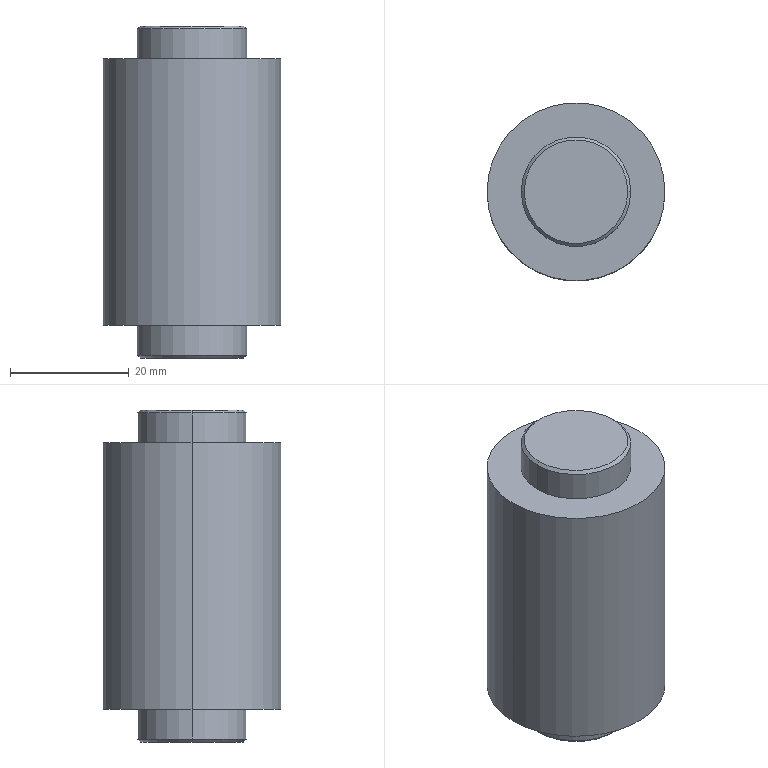Part | STEP file | CDAN75-Mbe | 1 solid | 14 faces | box 30 x 30 x 56 mm | volume 34751 mm3 | cylinder 6 | cone 4 | plane 4 | commonest cylinder face diameters 18.5 x4 30 x2
STEP:
#1=CARTESIAN_POINT('',(0.,0.,0.));
#2=DIRECTION('',(0.,0.,1.));
#3=DIRECTION('',(1.,0.,0.));
#4=AXIS2_PLACEMENT_3D('',#1,#2,#3);
#5=CARTESIAN_POINT('',(-71.,-59.,22.5));
#6=VERTEX_POINT('',#5);
#7=CARTESIAN_POINT('',(-41.,-59.,22.5));
#8=VERTEX_POINT('',#7);
#9=CARTESIAN_POINT('',(-56.,-59.,22.5));
#10=DIRECTION('',(0.,0.,-1.));
#11=DIRECTION('',(-1.,0.,0.));
#12=AXIS2_PLACEMENT_3D('',#9,#10,#11);
#13=CIRCLE('',#12,15.);
#14=CARTESIAN_POINT('',(-56.,-59.,0.));
#15=DIRECTION('',(0.,0.,-1.));
#16=DIRECTION('',(-1.,0.,0.));
#17=AXIS2_PLACEMENT_3D('',#14,#15,#16);
#18=CYLINDRICAL_SURFACE('',#17,15.);
#19=CARTESIAN_POINT('',(0.,-22.5));
#20=DIRECTION('',(1.,0.));
#21=VECTOR('',#20,1.);
#22=LINE('',#19,#21);
#23=(GEOMETRIC_REPRESENTATION_CONTEXT(2)PARAMETRIC_REPRESENTATION_CONTEXT()REPRESENTATION_CONTEXT('',''));
#24=DEFINITIONAL_REPRESENTATION('',(#22),#23);
#25=PCURVE('',#18,#24);
#26=CARTESIAN_POINT('',(-56.,-71.125,22.5));
#27=DIRECTION('',(0.,0.,1.));
#28=DIRECTION('',(1.,0.,0.));
#29=AXIS2_PLACEMENT_3D('',#26,#27,#28);
#30=PLANE('',#29);
#31=CARTESIAN_POINT('',(-15.,12.125));
#32=CARTESIAN_POINT('',(-15.,38.106));
#33=CARTESIAN_POINT('',(7.5,25.115));
#34=CARTESIAN_POINT('',(30.,12.125));
#35=CARTESIAN_POINT('',(7.5,-0.8654));
#36=CARTESIAN_POINT('',(-15.,-13.856));
#37=CARTESIAN_POINT('',(-15.,12.125));
#38=(BOUNDED_CURVE()B_SPLINE_CURVE(2,(#31,#32,#33,#34,#35,#36,#37),.UNSPECIFIED.,.T.,.F.)B_SPLINE_CURVE_WITH_KNOTS((1,2,2,2,2,1),(-2.094,0.,2.094,4.189,6.283,8.378),.UNSPECIFIED.)CURVE()GEOMETRIC_REPRESENTATION_ITEM()RATIONAL_B_SPLINE_CURVE((1.,0.5,1.,0.5,1.,0.5,1.))REPRESENTATION_ITEM(''));
#39=(GEOMETRIC_REPRESENTATION_CONTEXT(2)PARAMETRIC_REPRESENTATION_CONTEXT()REPRESENTATION_CONTEXT('',''));
#40=DEFINITIONAL_REPRESENTATION('',(#38),#39);
#41=PCURVE('',#30,#40);
#42=SURFACE_CURVE('',#13,(#25,#41),.PCURVE_S1.);
#43=EDGE_CURVE('',#6,#8,#42,.T.);
#44=ORIENTED_EDGE('',*,*,#43,.T.);
#45=CARTESIAN_POINT('',(-41.,-59.,-22.5));
#46=VERTEX_POINT('',#45);
#47=CARTESIAN_POINT('',(-41.,-59.,0.));
#48=DIRECTION('',(0.,0.,-1.));
#49=VECTOR('',#48,1.);
#50=LINE('',#47,#49);
#51=CARTESIAN_POINT('',(3.142,0.));
#52=DIRECTION('',(0.,1.));
#53=VECTOR('',#52,1.);
#54=LINE('',#51,#53);
#55=(GEOMETRIC_REPRESENTATION_CONTEXT(2)PARAMETRIC_REPRESENTATION_CONTEXT()REPRESENTATION_CONTEXT('',''));
#56=DEFINITIONAL_REPRESENTATION('',(#54),#55);
#57=PCURVE('',#18,#56);
#58=CARTESIAN_POINT('',(-56.,-59.,0.));
#59=DIRECTION('',(0.,0.,-1.));
#60=DIRECTION('',(-1.,0.,0.));
#61=AXIS2_PLACEMENT_3D('',#58,#59,#60);
#62=CYLINDRICAL_SURFACE('',#61,15.);
#63=CARTESIAN_POINT('',(3.142,0.));
#64=DIRECTION('',(0.,1.));
#65=VECTOR('',#64,1.);
#66=LINE('',#63,#65);
#67=(GEOMETRIC_REPRESENTATION_CONTEXT(2)PARAMETRIC_REPRESENTATION_CONTEXT()REPRESENTATION_CONTEXT('',''));
#68=DEFINITIONAL_REPRESENTATION('',(#66),#67);
#69=PCURVE('',#62,#68);
#70=SURFACE_CURVE('',#50,(#57,#69),.PCURVE_S1.);
#71=EDGE_CURVE('',#8,#46,#70,.T.);
#72=ORIENTED_EDGE('',*,*,#71,.T.);
#73=CARTESIAN_POINT('',(-71.,-59.,-22.5));
#74=VERTEX_POINT('',#73);
#75=CARTESIAN_POINT('',(-56.,-59.,-22.5));
#76=DIRECTION('',(0.,0.,1.));
#77=DIRECTION('',(-1.,0.,0.));
#78=AXIS2_PLACEMENT_3D('',#75,#76,#77);
#79=CIRCLE('',#78,15.);
#80=CARTESIAN_POINT('',(6.283,22.5));
#81=DIRECTION('',(-1.,0.));
#82=VECTOR('',#81,1.);
#83=LINE('',#80,#82);
#84=(GEOMETRIC_REPRESENTATION_CONTEXT(2)PARAMETRIC_REPRESENTATION_CONTEXT()REPRESENTATION_CONTEXT('',''));
#85=DEFINITIONAL_REPRESENTATION('',(#83),#84);
#86=PCURVE('',#18,#85);
#87=CARTESIAN_POINT('',(-56.,-71.125,-22.5));
#88=DIRECTION('',(0.,0.,-1.));
#89=DIRECTION('',(-1.,0.,0.));
#90=AXIS2_PLACEMENT_3D('',#87,#88,#89);
#91=PLANE('',#90);
#92=CARTESIAN_POINT('',(15.,12.125));
#93=CARTESIAN_POINT('',(15.,-13.856));
#94=CARTESIAN_POINT('',(-7.5,-0.8654));
#95=CARTESIAN_POINT('',(-30.,12.125));
#96=CARTESIAN_POINT('',(-7.5,25.115));
#97=CARTESIAN_POINT('',(15.,38.106));
#98=CARTESIAN_POINT('',(15.,12.125));
#99=(BOUNDED_CURVE()B_SPLINE_CURVE(2,(#92,#93,#94,#95,#96,#97,#98),.UNSPECIFIED.,.T.,.F.)B_SPLINE_CURVE_WITH_KNOTS((1,2,2,2,2,1),(-2.094,0.,2.094,4.189,6.283,8.378),.UNSPECIFIED.)CURVE()GEOMETRIC_REPRESENTATION_ITEM()RATIONAL_B_SPLINE_CURVE((1.,0.5,1.,0.5,1.,0.5,1.))REPRESENTATION_ITEM(''));
#100=(GEOMETRIC_REPRESENTATION_CONTEXT(2)PARAMETRIC_REPRESENTATION_CONTEXT()REPRESENTATION_CONTEXT('',''));
#101=DEFINITIONAL_REPRESENTATION('',(#99),#100);
#102=PCURVE('',#91,#101);
#103=SURFACE_CURVE('',#79,(#86,#102),.PCURVE_S1.);
#104=EDGE_CURVE('',#46,#74,#103,.T.);
#105=ORIENTED_EDGE('',*,*,#104,.T.);
#106=CARTESIAN_POINT('',(-71.,-59.,0.));
#107=DIRECTION('',(0.,0.,-1.));
#108=VECTOR('',#107,1.);
#109=LINE('',#106,#108);
#110=CARTESIAN_POINT('',(0.,0.));
#111=DIRECTION('',(0.,1.));
#112=VECTOR('',#111,1.);
#113=LINE('',#110,#112);
#114=(GEOMETRIC_REPRESENTATION_CONTEXT(2)PARAMETRIC_REPRESENTATION_CONTEXT()REPRESENTATION_CONTEXT('',''));
#115=DEFINITIONAL_REPRESENTATION('',(#113),#114);
#116=PCURVE('',#18,#115);
#117=CARTESIAN_POINT('',(6.283,0.));
#118=DIRECTION('',(0.,1.));
#119=VECTOR('',#118,1.);
#120=LINE('',#117,#119);
#121=(GEOMETRIC_REPRESENTATION_CONTEXT(2)PARAMETRIC_REPRESENTATION_CONTEXT()REPRESENTATION_CONTEXT('',''));
#122=DEFINITIONAL_REPRESENTATION('',(#120),#121);
#123=PCURVE('',#62,#122);
#124=SURFACE_CURVE('',#109,(#116,#123),.PCURVE_S1.);
#125=EDGE_CURVE('',#6,#74,#124,.T.);
#126=ORIENTED_EDGE('',*,*,#125,.F.);
#127=EDGE_LOOP('',(#44,#72,#105,#126));
#128=FACE_BOUND('',#127,.T.);
#129=ADVANCED_FACE('',(#128),#18,.T.);
#130=CARTESIAN_POINT('',(-46.75,-59.,-22.5));
#131=VERTEX_POINT('',#130);
#132=CARTESIAN_POINT('',(-65.25,-59.,-22.5));
#133=VERTEX_POINT('',#132);
#134=CARTESIAN_POINT('',(-56.,-59.,-22.5));
#135=DIRECTION('',(0.,0.,1.));
#136=DIRECTION('',(-1.,0.,0.));
#137=AXIS2_PLACEMENT_3D('',#134,#135,#136);
#138=CIRCLE('',#137,9.25);
#139=CARTESIAN_POINT('',(-56.,-59.,-25.));
#140=DIRECTION('',(0.,0.,-1.));
#141=DIRECTION('',(-1.,0.,0.));
#142=AXIS2_PLACEMENT_3D('',#139,#140,#141);
#143=CYLINDRICAL_SURFACE('',#142,9.25);
#144=CARTESIAN_POINT('',(6.283,-2.5));
#145=DIRECTION('',(-1.,0.));
#146=VECTOR('',#145,1.);
#147=LINE('',#144,#146);
#148=(GEOMETRIC_REPRESENTATION_CONTEXT(2)PARAMETRIC_REPRESENTATION_CONTEXT()REPRESENTATION_CONTEXT('',''));
#149=DEFINITIONAL_REPRESENTATION('',(#147),#148);
#150=PCURVE('',#143,#149);
#151=CARTESIAN_POINT('',(9.25,12.125));
#152=CARTESIAN_POINT('',(9.25,-3.896));
#153=CARTESIAN_POINT('',(-4.625,4.114));
#154=CARTESIAN_POINT('',(-18.5,12.125));
#155=CARTESIAN_POINT('',(-4.625,20.136));
#156=CARTESIAN_POINT('',(9.25,28.146));
#157=CARTESIAN_POINT('',(9.25,12.125));
#158=(BOUNDED_CURVE()B_SPLINE_CURVE(2,(#151,#152,#153,#154,#155,#156,#157),.UNSPECIFIED.,.T.,.F.)B_SPLINE_CURVE_WITH_KNOTS((1,2,2,2,2,1),(-2.094,0.,2.094,4.189,6.283,8.378),.UNSPECIFIED.)CURVE()GEOMETRIC_REPRESENTATION_ITEM()RATIONAL_B_SPLINE_CURVE((1.,0.5,1.,0.5,1.,0.5,1.))REPRESENTATION_ITEM(''));
#159=(GEOMETRIC_REPRESENTATION_CONTEXT(2)PARAMETRIC_REPRESENTATION_CONTEXT()REPRESENTATION_CONTEXT('',''));
#160=DEFINITIONAL_REPRESENTATION('',(#158),#159);
#161=PCURVE('',#91,#160);
#162=SURFACE_CURVE('',#138,(#150,#161),.PCURVE_S1.);
#163=EDGE_CURVE('',#131,#133,#162,.T.);
#164=ORIENTED_EDGE('',*,*,#163,.F.);
#165=CARTESIAN_POINT('',(-46.75,-59.,-27.5));
#166=VERTEX_POINT('',#165);
#167=CARTESIAN_POINT('',(-46.75,-59.,-25.));
#168=DIRECTION('',(0.,0.,-1.));
#169=VECTOR('',#168,1.);
#170=LINE('',#167,#169);
#171=CARTESIAN_POINT('',(3.142,0.));
#172=DIRECTION('',(0.,1.));
#173=VECTOR('',#172,1.);
#174=LINE('',#171,#173);
#175=(GEOMETRIC_REPRESENTATION_CONTEXT(2)PARAMETRIC_REPRESENTATION_CONTEXT()REPRESENTATION_CONTEXT('',''));
#176=DEFINITIONAL_REPRESENTATION('',(#174),#175);
#177=PCURVE('',#143,#176);
#178=CARTESIAN_POINT('',(-56.,-59.,-25.));
#179=DIRECTION('',(0.,0.,-1.));
#180=DIRECTION('',(-1.,0.,0.));
#181=AXIS2_PLACEMENT_3D('',#178,#179,#180);
#182=CYLINDRICAL_SURFACE('',#181,9.25);
#183=CARTESIAN_POINT('',(3.142,0.));
#184=DIRECTION('',(0.,1.));
#185=VECTOR('',#184,1.);
#186=LINE('',#183,#185);
#187=(GEOMETRIC_REPRESENTATION_CONTEXT(2)PARAMETRIC_REPRESENTATION_CONTEXT()REPRESENTATION_CONTEXT('',''));
#188=DEFINITIONAL_REPRESENTATION('',(#186),#187);
#189=PCURVE('',#182,#188);
#190=SURFACE_CURVE('',#170,(#177,#189),.PCURVE_S1.);
#191=EDGE_CURVE('',#131,#166,#190,.T.);
#192=ORIENTED_EDGE('',*,*,#191,.T.);
#193=CARTESIAN_POINT('',(-65.25,-59.,-27.5));
#194=VERTEX_POINT('',#193);
#195=CARTESIAN_POINT('',(-56.,-59.,-27.5));
#196=DIRECTION('',(0.,0.,1.));
#197=DIRECTION('',(-1.,0.,0.));
#198=AXIS2_PLACEMENT_3D('',#195,#196,#197);
#199=CIRCLE('',#198,9.25);
#200=CARTESIAN_POINT('',(6.283,2.5));
#201=DIRECTION('',(-1.,0.));
#202=VECTOR('',#201,1.);
#203=LINE('',#200,#202);
#204=(GEOMETRIC_REPRESENTATION_CONTEXT(2)PARAMETRIC_REPRESENTATION_CONTEXT()REPRESENTATION_CONTEXT('',''));
#205=DEFINITIONAL_REPRESENTATION('',(#203),#204);
#206=PCURVE('',#143,#205);
#207=CARTESIAN_POINT('',(-56.,-59.,-27.5));
#208=DIRECTION('',(0.,0.,1.));
#209=DIRECTION('',(1.,0.,0.));
#210=AXIS2_PLACEMENT_3D('',#207,#208,#209);
#211=CONICAL_SURFACE('',#210,9.25,0.7854);
#212=CARTESIAN_POINT('',(-3.142,0.));
#213=DIRECTION('',(1.,0.));
#214=VECTOR('',#213,1.);
#215=LINE('',#212,#214);
#216=(GEOMETRIC_REPRESENTATION_CONTEXT(2)PARAMETRIC_REPRESENTATION_CONTEXT()REPRESENTATION_CONTEXT('',''));
#217=DEFINITIONAL_REPRESENTATION('',(#215),#216);
#218=PCURVE('',#211,#217);
#219=SURFACE_CURVE('',#199,(#206,#218),.PCURVE_S1.);
#220=EDGE_CURVE('',#166,#194,#219,.T.);
#221=ORIENTED_EDGE('',*,*,#220,.T.);
#222=CARTESIAN_POINT('',(-65.25,-59.,-25.));
#223=DIRECTION('',(0.,0.,-1.));
#224=VECTOR('',#223,1.);
#225=LINE('',#222,#224);
#226=CARTESIAN_POINT('',(0.,0.));
#227=DIRECTION('',(0.,1.));
#228=VECTOR('',#227,1.);
#229=LINE('',#226,#228);
#230=(GEOMETRIC_REPRESENTATION_CONTEXT(2)PARAMETRIC_REPRESENTATION_CONTEXT()REPRESENTATION_CONTEXT('',''));
#231=DEFINITIONAL_REPRESENTATION('',(#229),#230);
#232=PCURVE('',#143,#231);
#233=CARTESIAN_POINT('',(6.283,0.));
#234=DIRECTION('',(0.,1.));
#235=VECTOR('',#234,1.);
#236=LINE('',#233,#235);
#237=(GEOMETRIC_REPRESENTATION_CONTEXT(2)PARAMETRIC_REPRESENTATION_CONTEXT()REPRESENTATION_CONTEXT('',''));
#238=DEFINITIONAL_REPRESENTATION('',(#236),#237);
#239=PCURVE('',#182,#238);
#240=SURFACE_CURVE('',#225,(#232,#239),.PCURVE_S1.);
#241=EDGE_CURVE('',#133,#194,#240,.T.);
#242=ORIENTED_EDGE('',*,*,#241,.F.);
#243=EDGE_LOOP('',(#164,#192,#221,#242));
#244=FACE_BOUND('',#243,.T.);
#245=ADVANCED_FACE('',(#244),#143,.T.);
#246=CARTESIAN_POINT('',(-65.25,-59.,27.5));
#247=VERTEX_POINT('',#246);
#248=CARTESIAN_POINT('',(-46.75,-59.,27.5));
#249=VERTEX_POINT('',#248);
#250=CARTESIAN_POINT('',(-56.,-59.,27.5));
#251=DIRECTION('',(0.,0.,-1.));
#252=DIRECTION('',(-1.,0.,0.));
#253=AXIS2_PLACEMENT_3D('',#250,#251,#252);
#254=CIRCLE('',#253,9.25);
#255=CARTESIAN_POINT('',(-56.,-59.,25.));
#256=DIRECTION('',(0.,0.,-1.));
#257=DIRECTION('',(-1.,0.,0.));
#258=AXIS2_PLACEMENT_3D('',#255,#256,#257);
#259=CYLINDRICAL_SURFACE('',#258,9.25);
#260=CARTESIAN_POINT('',(0.,-2.5));
#261=DIRECTION('',(1.,0.));
#262=VECTOR('',#261,1.);
#263=LINE('',#260,#262);
#264=(GEOMETRIC_REPRESENTATION_CONTEXT(2)PARAMETRIC_REPRESENTATION_CONTEXT()REPRESENTATION_CONTEXT('',''));
#265=DEFINITIONAL_REPRESENTATION('',(#263),#264);
#266=PCURVE('',#259,#265);
#267=CARTESIAN_POINT('',(-56.,-59.,27.5));
#268=DIRECTION('',(0.,0.,-1.));
#269=DIRECTION('',(-1.,0.,0.));
#270=AXIS2_PLACEMENT_3D('',#267,#268,#269);
#271=CONICAL_SURFACE('',#270,9.25,0.7854);
#272=CARTESIAN_POINT('',(0.,0.));
#273=DIRECTION('',(1.,0.));
#274=VECTOR('',#273,1.);
#275=LINE('',#272,#274);
#276=(GEOMETRIC_REPRESENTATION_CONTEXT(2)PARAMETRIC_REPRESENTATION_CONTEXT()REPRESENTATION_CONTEXT('',''));
#277=DEFINITIONAL_REPRESENTATION('',(#275),#276);
#278=PCURVE('',#271,#277);
#279=SURFACE_CURVE('',#254,(#266,#278),.PCURVE_S1.);
#280=EDGE_CURVE('',#247,#249,#279,.T.);
#281=ORIENTED_EDGE('',*,*,#280,.T.);
#282=CARTESIAN_POINT('',(-46.75,-59.,22.5));
#283=VERTEX_POINT('',#282);
#284=CARTESIAN_POINT('',(-46.75,-59.,25.));
#285=DIRECTION('',(0.,0.,-1.));
#286=VECTOR('',#285,1.);
#287=LINE('',#284,#286);
#288=CARTESIAN_POINT('',(3.142,0.));
#289=DIRECTION('',(0.,1.));
#290=VECTOR('',#289,1.);
#291=LINE('',#288,#290);
#292=(GEOMETRIC_REPRESENTATION_CONTEXT(2)PARAMETRIC_REPRESENTATION_CONTEXT()REPRESENTATION_CONTEXT('',''));
#293=DEFINITIONAL_REPRESENTATION('',(#291),#292);
#294=PCURVE('',#259,#293);
#295=CARTESIAN_POINT('',(-56.,-59.,25.));
#296=DIRECTION('',(0.,0.,-1.));
#297=DIRECTION('',(-1.,0.,0.));
#298=AXIS2_PLACEMENT_3D('',#295,#296,#297);
#299=CYLINDRICAL_SURFACE('',#298,9.25);
#300=CARTESIAN_POINT('',(3.142,0.));
#301=DIRECTION('',(0.,1.));
#302=VECTOR('',#301,1.);
#303=LINE('',#300,#302);
#304=(GEOMETRIC_REPRESENTATION_CONTEXT(2)PARAMETRIC_REPRESENTATION_CONTEXT()REPRESENTATION_CONTEXT('',''));
#305=DEFINITIONAL_REPRESENTATION('',(#303),#304);
#306=PCURVE('',#299,#305);
#307=SURFACE_CURVE('',#287,(#294,#306),.PCURVE_S1.);
#308=EDGE_CURVE('',#249,#283,#307,.T.);
#309=ORIENTED_EDGE('',*,*,#308,.T.);
#310=CARTESIAN_POINT('',(-65.25,-59.,22.5));
#311=VERTEX_POINT('',#310);
#312=CARTESIAN_POINT('',(-56.,-59.,22.5));
#313=DIRECTION('',(0.,0.,-1.));
#314=DIRECTION('',(-1.,0.,0.));
#315=AXIS2_PLACEMENT_3D('',#312,#313,#314);
#316=CIRCLE('',#315,9.25);
#317=CARTESIAN_POINT('',(0.,2.5));
#318=DIRECTION('',(1.,0.));
#319=VECTOR('',#318,1.);
#320=LINE('',#317,#319);
#321=(GEOMETRIC_REPRESENTATION_CONTEXT(2)PARAMETRIC_REPRESENTATION_CONTEXT()REPRESENTATION_CONTEXT('',''));
#322=DEFINITIONAL_REPRESENTATION('',(#320),#321);
#323=PCURVE('',#259,#322);
#324=CARTESIAN_POINT('',(-9.25,12.125));
#325=CARTESIAN_POINT('',(-9.25,28.146));
#326=CARTESIAN_POINT('',(4.625,20.136));
#327=CARTESIAN_POINT('',(18.5,12.125));
#328=CARTESIAN_POINT('',(4.625,4.114));
#329=CARTESIAN_POINT('',(-9.25,-3.896));
#330=CARTESIAN_POINT('',(-9.25,12.125));
#331=(BOUNDED_CURVE()B_SPLINE_CURVE(2,(#324,#325,#326,#327,#328,#329,#330),.UNSPECIFIED.,.T.,.F.)B_SPLINE_CURVE_WITH_KNOTS((1,2,2,2,2,1),(-2.094,0.,2.094,4.189,6.283,8.378),.UNSPECIFIED.)CURVE()GEOMETRIC_REPRESENTATION_ITEM()RATIONAL_B_SPLINE_CURVE((1.,0.5,1.,0.5,1.,0.5,1.))REPRESENTATION_ITEM(''));
#332=(GEOMETRIC_REPRESENTATION_CONTEXT(2)PARAMETRIC_REPRESENTATION_CONTEXT()REPRESENTATION_CONTEXT('',''));
#333=DEFINITIONAL_REPRESENTATION('',(#331),#332);
#334=PCURVE('',#30,#333);
#335=SURFACE_CURVE('',#316,(#323,#334),.PCURVE_S1.);
#336=EDGE_CURVE('',#311,#283,#335,.T.);
#337=ORIENTED_EDGE('',*,*,#336,.F.);
#338=CARTESIAN_POINT('',(-65.25,-59.,25.));
#339=DIRECTION('',(0.,0.,-1.));
#340=VECTOR('',#339,1.);
#341=LINE('',#338,#340);
#342=CARTESIAN_POINT('',(0.,0.));
#343=DIRECTION('',(0.,1.));
#344=VECTOR('',#343,1.);
#345=LINE('',#342,#344);
#346=(GEOMETRIC_REPRESENTATION_CONTEXT(2)PARAMETRIC_REPRESENTATION_CONTEXT()REPRESENTATION_CONTEXT('',''));
#347=DEFINITIONAL_REPRESENTATION('',(#345),#346);
#348=PCURVE('',#259,#347);
#349=CARTESIAN_POINT('',(6.283,0.));
#350=DIRECTION('',(0.,1.));
#351=VECTOR('',#350,1.);
#352=LINE('',#349,#351);
#353=(GEOMETRIC_REPRESENTATION_CONTEXT(2)PARAMETRIC_REPRESENTATION_CONTEXT()REPRESENTATION_CONTEXT('',''));
#354=DEFINITIONAL_REPRESENTATION('',(#352),#353);
#355=PCURVE('',#299,#354);
#356=SURFACE_CURVE('',#341,(#348,#355),.PCURVE_S1.);
#357=EDGE_CURVE('',#247,#311,#356,.T.);
#358=ORIENTED_EDGE('',*,*,#357,.F.);
#359=EDGE_LOOP('',(#281,#309,#337,#358));
#360=FACE_BOUND('',#359,.T.);
#361=ADVANCED_FACE('',(#360),#259,.T.);
#362=CARTESIAN_POINT('',(-47.25,-59.,-28.));
#363=VERTEX_POINT('',#362);
#364=CARTESIAN_POINT('',(-64.75,-59.,-28.));
#365=VERTEX_POINT('',#364);
#366=CARTESIAN_POINT('',(-56.,-59.,-28.));
#367=DIRECTION('',(0.,0.,1.));
#368=DIRECTION('',(1.,0.,0.));
#369=AXIS2_PLACEMENT_3D('',#366,#367,#368);
#370=CIRCLE('',#369,8.75);
#371=CARTESIAN_POINT('',(0.,-0.5));
#372=DIRECTION('',(1.,0.));
#373=VECTOR('',#372,1.);
#374=LINE('',#371,#373);
#375=(GEOMETRIC_REPRESENTATION_CONTEXT(2)PARAMETRIC_REPRESENTATION_CONTEXT()REPRESENTATION_CONTEXT('',''));
#376=DEFINITIONAL_REPRESENTATION('',(#374),#375);
#377=PCURVE('',#211,#376);
#378=CARTESIAN_POINT('',(-56.,-63.375,-28.));
#379=DIRECTION('',(0.,0.,-1.));
#380=DIRECTION('',(-1.,0.,0.));
#381=AXIS2_PLACEMENT_3D('',#378,#379,#380);
#382=PLANE('',#381);
#383=CARTESIAN_POINT('',(-8.75,4.375));
#384=CARTESIAN_POINT('',(-8.75,19.53));
#385=CARTESIAN_POINT('',(4.375,11.953));
#386=CARTESIAN_POINT('',(17.5,4.375));
#387=CARTESIAN_POINT('',(4.375,-3.203));
#388=CARTESIAN_POINT('',(-8.75,-10.78));
#389=CARTESIAN_POINT('',(-8.75,4.375));
#390=(BOUNDED_CURVE()B_SPLINE_CURVE(2,(#383,#384,#385,#386,#387,#388,#389),.UNSPECIFIED.,.T.,.F.)B_SPLINE_CURVE_WITH_KNOTS((1,2,2,2,2,1),(-2.094,0.,2.094,4.189,6.283,8.378),.UNSPECIFIED.)CURVE()GEOMETRIC_REPRESENTATION_ITEM()RATIONAL_B_SPLINE_CURVE((1.,0.5,1.,0.5,1.,0.5,1.))REPRESENTATION_ITEM(''));
#391=(GEOMETRIC_REPRESENTATION_CONTEXT(2)PARAMETRIC_REPRESENTATION_CONTEXT()REPRESENTATION_CONTEXT('',''));
#392=DEFINITIONAL_REPRESENTATION('',(#390),#391);
#393=PCURVE('',#382,#392);
#394=SURFACE_CURVE('',#370,(#377,#393),.PCURVE_S1.);
#395=EDGE_CURVE('',#363,#365,#394,.T.);
#396=ORIENTED_EDGE('',*,*,#395,.T.);
#397=CARTESIAN_POINT('',(-65.25,-59.,-27.5));
#398=DIRECTION('',(-0.7071,0.,0.7071));
#399=VECTOR('',#398,1.);
#400=LINE('',#397,#399);
#401=CARTESIAN_POINT('',(3.142,0.));
#402=DIRECTION('',(0.,1.));
#403=VECTOR('',#402,1.);
#404=LINE('',#401,#403);
#405=(GEOMETRIC_REPRESENTATION_CONTEXT(2)PARAMETRIC_REPRESENTATION_CONTEXT()REPRESENTATION_CONTEXT('',''));
#406=DEFINITIONAL_REPRESENTATION('',(#404),#405);
#407=PCURVE('',#211,#406);
#408=CARTESIAN_POINT('',(-56.,-59.,-27.5));
#409=DIRECTION('',(0.,0.,1.));
#410=DIRECTION('',(1.,0.,0.));
#411=AXIS2_PLACEMENT_3D('',#408,#409,#410);
#412=CONICAL_SURFACE('',#411,9.25,0.7854);
#413=CARTESIAN_POINT('',(3.142,0.));
#414=DIRECTION('',(0.,1.));
#415=VECTOR('',#414,1.);
#416=LINE('',#413,#415);
#417=(GEOMETRIC_REPRESENTATION_CONTEXT(2)PARAMETRIC_REPRESENTATION_CONTEXT()REPRESENTATION_CONTEXT('',''));
#418=DEFINITIONAL_REPRESENTATION('',(#416),#417);
#419=PCURVE('',#412,#418);
#420=SURFACE_CURVE('',#400,(#407,#419),.PCURVE_S1.);
#421=EDGE_CURVE('',#365,#194,#420,.T.);
#422=ORIENTED_EDGE('',*,*,#421,.T.);
#423=ORIENTED_EDGE('',*,*,#220,.F.);
#424=CARTESIAN_POINT('',(-46.75,-59.,-27.5));
#425=DIRECTION('',(0.7071,0.,0.7071));
#426=VECTOR('',#425,1.);
#427=LINE('',#424,#426);
#428=CARTESIAN_POINT('',(0.,0.));
#429=DIRECTION('',(0.,1.));
#430=VECTOR('',#429,1.);
#431=LINE('',#428,#430);
#432=(GEOMETRIC_REPRESENTATION_CONTEXT(2)PARAMETRIC_REPRESENTATION_CONTEXT()REPRESENTATION_CONTEXT('',''));
#433=DEFINITIONAL_REPRESENTATION('',(#431),#432);
#434=PCURVE('',#211,#433);
#435=CARTESIAN_POINT('',(6.283,0.));
#436=DIRECTION('',(0.,1.));
#437=VECTOR('',#436,1.);
#438=LINE('',#435,#437);
#439=(GEOMETRIC_REPRESENTATION_CONTEXT(2)PARAMETRIC_REPRESENTATION_CONTEXT()REPRESENTATION_CONTEXT('',''));
#440=DEFINITIONAL_REPRESENTATION('',(#438),#439);
#441=PCURVE('',#412,#440);
#442=SURFACE_CURVE('',#427,(#434,#441),.PCURVE_S1.);
#443=EDGE_CURVE('',#363,#166,#442,.T.);
#444=ORIENTED_EDGE('',*,*,#443,.F.);
#445=EDGE_LOOP('',(#396,#422,#423,#444));
#446=FACE_BOUND('',#445,.T.);
#447=ADVANCED_FACE('',(#446),#211,.T.);
#448=CARTESIAN_POINT('',(-64.75,-59.,28.));
#449=VERTEX_POINT('',#448);
#450=CARTESIAN_POINT('',(-47.25,-59.,28.));
#451=VERTEX_POINT('',#450);
#452=CARTESIAN_POINT('',(-56.,-59.,28.));
#453=DIRECTION('',(0.,0.,-1.));
#454=DIRECTION('',(-1.,0.,0.));
#455=AXIS2_PLACEMENT_3D('',#452,#453,#454);
#456=CIRCLE('',#455,8.75);
#457=CARTESIAN_POINT('',(0.,-0.5));
#458=DIRECTION('',(1.,0.));
#459=VECTOR('',#458,1.);
#460=LINE('',#457,#459);
#461=(GEOMETRIC_REPRESENTATION_CONTEXT(2)PARAMETRIC_REPRESENTATION_CONTEXT()REPRESENTATION_CONTEXT('',''));
#462=DEFINITIONAL_REPRESENTATION('',(#460),#461);
#463=PCURVE('',#271,#462);
#464=CARTESIAN_POINT('',(-56.,-63.375,28.));
#465=DIRECTION('',(0.,0.,1.));
#466=DIRECTION('',(1.,0.,0.));
#467=AXIS2_PLACEMENT_3D('',#464,#465,#466);
#468=PLANE('',#467);
#469=CARTESIAN_POINT('',(-8.75,4.375));
#470=CARTESIAN_POINT('',(-8.75,19.53));
#471=CARTESIAN_POINT('',(4.375,11.953));
#472=CARTESIAN_POINT('',(17.5,4.375));
#473=CARTESIAN_POINT('',(4.375,-3.203));
#474=CARTESIAN_POINT('',(-8.75,-10.78));
#475=CARTESIAN_POINT('',(-8.75,4.375));
#476=(BOUNDED_CURVE()B_SPLINE_CURVE(2,(#469,#470,#471,#472,#473,#474,#475),.UNSPECIFIED.,.T.,.F.)B_SPLINE_CURVE_WITH_KNOTS((1,2,2,2,2,1),(-2.094,0.,2.094,4.189,6.283,8.378),.UNSPECIFIED.)CURVE()GEOMETRIC_REPRESENTATION_ITEM()RATIONAL_B_SPLINE_CURVE((1.,0.5,1.,0.5,1.,0.5,1.))REPRESENTATION_ITEM(''));
#477=(GEOMETRIC_REPRESENTATION_CONTEXT(2)PARAMETRIC_REPRESENTATION_CONTEXT()REPRESENTATION_CONTEXT('',''));
#478=DEFINITIONAL_REPRESENTATION('',(#476),#477);
#479=PCURVE('',#468,#478);
#480=SURFACE_CURVE('',#456,(#463,#479),.PCURVE_S1.);
#481=EDGE_CURVE('',#449,#451,#480,.T.);
#482=ORIENTED_EDGE('',*,*,#481,.T.);
#483=CARTESIAN_POINT('',(-46.75,-59.,27.5));
#484=DIRECTION('',(0.7071,0.,-0.7071));
#485=VECTOR('',#484,1.);
#486=LINE('',#483,#485);
#487=CARTESIAN_POINT('',(3.142,0.));
#488=DIRECTION('',(0.,1.));
#489=VECTOR('',#488,1.);
#490=LINE('',#487,#489);
#491=(GEOMETRIC_REPRESENTATION_CONTEXT(2)PARAMETRIC_REPRESENTATION_CONTEXT()REPRESENTATION_CONTEXT('',''));
#492=DEFINITIONAL_REPRESENTATION('',(#490),#491);
#493=PCURVE('',#271,#492);
#494=CARTESIAN_POINT('',(-56.,-59.,27.5));
#495=DIRECTION('',(0.,0.,-1.));
#496=DIRECTION('',(-1.,0.,0.));
#497=AXIS2_PLACEMENT_3D('',#494,#495,#496);
#498=CONICAL_SURFACE('',#497,9.25,0.7854);
#499=CARTESIAN_POINT('',(3.142,0.));
#500=DIRECTION('',(0.,1.));
#501=VECTOR('',#500,1.);
#502=LINE('',#499,#501);
#503=(GEOMETRIC_REPRESENTATION_CONTEXT(2)PARAMETRIC_REPRESENTATION_CONTEXT()REPRESENTATION_CONTEXT('',''));
#504=DEFINITIONAL_REPRESENTATION('',(#502),#503);
#505=PCURVE('',#498,#504);
#506=SURFACE_CURVE('',#486,(#493,#505),.PCURVE_S1.);
#507=EDGE_CURVE('',#451,#249,#506,.T.);
#508=ORIENTED_EDGE('',*,*,#507,.T.);
#509=ORIENTED_EDGE('',*,*,#280,.F.);
#510=CARTESIAN_POINT('',(-65.25,-59.,27.5));
#511=DIRECTION('',(-0.7071,0.,-0.7071));
#512=VECTOR('',#511,1.);
#513=LINE('',#510,#512);
#514=CARTESIAN_POINT('',(0.,0.));
#515=DIRECTION('',(0.,1.));
#516=VECTOR('',#515,1.);
#517=LINE('',#514,#516);
#518=(GEOMETRIC_REPRESENTATION_CONTEXT(2)PARAMETRIC_REPRESENTATION_CONTEXT()REPRESENTATION_CONTEXT('',''));
#519=DEFINITIONAL_REPRESENTATION('',(#517),#518);
#520=PCURVE('',#271,#519);
#521=CARTESIAN_POINT('',(6.283,0.));
#522=DIRECTION('',(0.,1.));
#523=VECTOR('',#522,1.);
#524=LINE('',#521,#523);
#525=(GEOMETRIC_REPRESENTATION_CONTEXT(2)PARAMETRIC_REPRESENTATION_CONTEXT()REPRESENTATION_CONTEXT('',''));
#526=DEFINITIONAL_REPRESENTATION('',(#524),#525);
#527=PCURVE('',#498,#526);
#528=SURFACE_CURVE('',#513,(#520,#527),.PCURVE_S1.);
#529=EDGE_CURVE('',#449,#247,#528,.T.);
#530=ORIENTED_EDGE('',*,*,#529,.F.);
#531=EDGE_LOOP('',(#482,#508,#509,#530));
#532=FACE_BOUND('',#531,.T.);
#533=ADVANCED_FACE('',(#532),#271,.T.);
#534=ORIENTED_EDGE('',*,*,#71,.F.);
#535=CARTESIAN_POINT('',(-56.,-59.,22.5));
#536=DIRECTION('',(0.,0.,-1.));
#537=DIRECTION('',(-1.,0.,0.));
#538=AXIS2_PLACEMENT_3D('',#535,#536,#537);
#539=CIRCLE('',#538,15.);
#540=CARTESIAN_POINT('',(0.,-22.5));
#541=DIRECTION('',(1.,0.));
#542=VECTOR('',#541,1.);
#543=LINE('',#540,#542);
#544=(GEOMETRIC_REPRESENTATION_CONTEXT(2)PARAMETRIC_REPRESENTATION_CONTEXT()REPRESENTATION_CONTEXT('',''));
#545=DEFINITIONAL_REPRESENTATION('',(#543),#544);
#546=PCURVE('',#62,#545);
#547=CARTESIAN_POINT('',(-15.,12.125));
#548=CARTESIAN_POINT('',(-15.,38.106));
#549=CARTESIAN_POINT('',(7.5,25.115));
#550=CARTESIAN_POINT('',(30.,12.125));
#551=CARTESIAN_POINT('',(7.5,-0.8654));
#552=CARTESIAN_POINT('',(-15.,-13.856));
#553=CARTESIAN_POINT('',(-15.,12.125));
#554=(BOUNDED_CURVE()B_SPLINE_CURVE(2,(#547,#548,#549,#550,#551,#552,#553),.UNSPECIFIED.,.T.,.F.)B_SPLINE_CURVE_WITH_KNOTS((1,2,2,2,2,1),(-2.094,0.,2.094,4.189,6.283,8.378),.UNSPECIFIED.)CURVE()GEOMETRIC_REPRESENTATION_ITEM()RATIONAL_B_SPLINE_CURVE((1.,0.5,1.,0.5,1.,0.5,1.))REPRESENTATION_ITEM(''));
#555=(GEOMETRIC_REPRESENTATION_CONTEXT(2)PARAMETRIC_REPRESENTATION_CONTEXT()REPRESENTATION_CONTEXT('',''));
#556=DEFINITIONAL_REPRESENTATION('',(#554),#555);
#557=PCURVE('',#30,#556);
#558=SURFACE_CURVE('',#539,(#546,#557),.PCURVE_S1.);
#559=EDGE_CURVE('',#8,#6,#558,.T.);
#560=ORIENTED_EDGE('',*,*,#559,.T.);
#561=ORIENTED_EDGE('',*,*,#125,.T.);
#562=CARTESIAN_POINT('',(-56.,-59.,-22.5));
#563=DIRECTION('',(0.,0.,1.));
#564=DIRECTION('',(-1.,0.,0.));
#565=AXIS2_PLACEMENT_3D('',#562,#563,#564);
#566=CIRCLE('',#565,15.);
#567=CARTESIAN_POINT('',(6.283,22.5));
#568=DIRECTION('',(-1.,0.));
#569=VECTOR('',#568,1.);
#570=LINE('',#567,#569);
#571=(GEOMETRIC_REPRESENTATION_CONTEXT(2)PARAMETRIC_REPRESENTATION_CONTEXT()REPRESENTATION_CONTEXT('',''));
#572=DEFINITIONAL_REPRESENTATION('',(#570),#571);
#573=PCURVE('',#62,#572);
#574=CARTESIAN_POINT('',(15.,12.125));
#575=CARTESIAN_POINT('',(15.,-13.856));
#576=CARTESIAN_POINT('',(-7.5,-0.8654));
#577=CARTESIAN_POINT('',(-30.,12.125));
#578=CARTESIAN_POINT('',(-7.5,25.115));
#579=CARTESIAN_POINT('',(15.,38.106));
#580=CARTESIAN_POINT('',(15.,12.125));
#581=(BOUNDED_CURVE()B_SPLINE_CURVE(2,(#574,#575,#576,#577,#578,#579,#580),.UNSPECIFIED.,.T.,.F.)B_SPLINE_CURVE_WITH_KNOTS((1,2,2,2,2,1),(-2.094,0.,2.094,4.189,6.283,8.378),.UNSPECIFIED.)CURVE()GEOMETRIC_REPRESENTATION_ITEM()RATIONAL_B_SPLINE_CURVE((1.,0.5,1.,0.5,1.,0.5,1.))REPRESENTATION_ITEM(''));
#582=(GEOMETRIC_REPRESENTATION_CONTEXT(2)PARAMETRIC_REPRESENTATION_CONTEXT()REPRESENTATION_CONTEXT('',''));
#583=DEFINITIONAL_REPRESENTATION('',(#581),#582);
#584=PCURVE('',#91,#583);
#585=SURFACE_CURVE('',#566,(#573,#584),.PCURVE_S1.);
#586=EDGE_CURVE('',#74,#46,#585,.T.);
#587=ORIENTED_EDGE('',*,*,#586,.T.);
#588=EDGE_LOOP('',(#534,#560,#561,#587));
#589=FACE_BOUND('',#588,.T.);
#590=ADVANCED_FACE('',(#589),#62,.T.);
#591=ORIENTED_EDGE('',*,*,#586,.F.);
#592=ORIENTED_EDGE('',*,*,#104,.F.);
#593=EDGE_LOOP('',(#591,#592));
#594=FACE_BOUND('',#593,.T.);
#595=CARTESIAN_POINT('',(-56.,-59.,-22.5));
#596=DIRECTION('',(0.,0.,1.));
#597=DIRECTION('',(-1.,0.,0.));
#598=AXIS2_PLACEMENT_3D('',#595,#596,#597);
#599=CIRCLE('',#598,9.25);
#600=CARTESIAN_POINT('',(9.25,12.125));
#601=CARTESIAN_POINT('',(9.25,-3.896));
#602=CARTESIAN_POINT('',(-4.625,4.114));
#603=CARTESIAN_POINT('',(-18.5,12.125));
#604=CARTESIAN_POINT('',(-4.625,20.136));
#605=CARTESIAN_POINT('',(9.25,28.146));
#606=CARTESIAN_POINT('',(9.25,12.125));
#607=(BOUNDED_CURVE()B_SPLINE_CURVE(2,(#600,#601,#602,#603,#604,#605,#606),.UNSPECIFIED.,.T.,.F.)B_SPLINE_CURVE_WITH_KNOTS((1,2,2,2,2,1),(-2.094,0.,2.094,4.189,6.283,8.378),.UNSPECIFIED.)CURVE()GEOMETRIC_REPRESENTATION_ITEM()RATIONAL_B_SPLINE_CURVE((1.,0.5,1.,0.5,1.,0.5,1.))REPRESENTATION_ITEM(''));
#608=(GEOMETRIC_REPRESENTATION_CONTEXT(2)PARAMETRIC_REPRESENTATION_CONTEXT()REPRESENTATION_CONTEXT('',''));
#609=DEFINITIONAL_REPRESENTATION('',(#607),#608);
#610=PCURVE('',#91,#609);
#611=CARTESIAN_POINT('',(6.283,-2.5));
#612=DIRECTION('',(-1.,0.));
#613=VECTOR('',#612,1.);
#614=LINE('',#611,#613);
#615=(GEOMETRIC_REPRESENTATION_CONTEXT(2)PARAMETRIC_REPRESENTATION_CONTEXT()REPRESENTATION_CONTEXT('',''));
#616=DEFINITIONAL_REPRESENTATION('',(#614),#615);
#617=PCURVE('',#182,#616);
#618=SURFACE_CURVE('',#599,(#610,#617),.PCURVE_S1.);
#619=EDGE_CURVE('',#133,#131,#618,.T.);
#620=ORIENTED_EDGE('',*,*,#619,.T.);
#621=ORIENTED_EDGE('',*,*,#163,.T.);
#622=EDGE_LOOP('',(#620,#621));
#623=FACE_BOUND('',#622,.T.);
#624=ADVANCED_FACE('',(#594,#623),#91,.T.);
#625=ORIENTED_EDGE('',*,*,#336,.T.);
#626=CARTESIAN_POINT('',(-56.,-59.,22.5));
#627=DIRECTION('',(0.,0.,-1.));
#628=DIRECTION('',(-1.,0.,0.));
#629=AXIS2_PLACEMENT_3D('',#626,#627,#628);
#630=CIRCLE('',#629,9.25);
#631=CARTESIAN_POINT('',(-9.25,12.125));
#632=CARTESIAN_POINT('',(-9.25,28.146));
#633=CARTESIAN_POINT('',(4.625,20.136));
#634=CARTESIAN_POINT('',(18.5,12.125));
#635=CARTESIAN_POINT('',(4.625,4.114));
#636=CARTESIAN_POINT('',(-9.25,-3.896));
#637=CARTESIAN_POINT('',(-9.25,12.125));
#638=(BOUNDED_CURVE()B_SPLINE_CURVE(2,(#631,#632,#633,#634,#635,#636,#637),.UNSPECIFIED.,.T.,.F.)B_SPLINE_CURVE_WITH_KNOTS((1,2,2,2,2,1),(-2.094,0.,2.094,4.189,6.283,8.378),.UNSPECIFIED.)CURVE()GEOMETRIC_REPRESENTATION_ITEM()RATIONAL_B_SPLINE_CURVE((1.,0.5,1.,0.5,1.,0.5,1.))REPRESENTATION_ITEM(''));
#639=(GEOMETRIC_REPRESENTATION_CONTEXT(2)PARAMETRIC_REPRESENTATION_CONTEXT()REPRESENTATION_CONTEXT('',''));
#640=DEFINITIONAL_REPRESENTATION('',(#638),#639);
#641=PCURVE('',#30,#640);
#642=CARTESIAN_POINT('',(0.,2.5));
#643=DIRECTION('',(1.,0.));
#644=VECTOR('',#643,1.);
#645=LINE('',#642,#644);
#646=(GEOMETRIC_REPRESENTATION_CONTEXT(2)PARAMETRIC_REPRESENTATION_CONTEXT()REPRESENTATION_CONTEXT('',''));
#647=DEFINITIONAL_REPRESENTATION('',(#645),#646);
#648=PCURVE('',#299,#647);
#649=SURFACE_CURVE('',#630,(#641,#648),.PCURVE_S1.);
#650=EDGE_CURVE('',#283,#311,#649,.T.);
#651=ORIENTED_EDGE('',*,*,#650,.T.);
#652=EDGE_LOOP('',(#625,#651));
#653=FACE_BOUND('',#652,.T.);
#654=ORIENTED_EDGE('',*,*,#43,.F.);
#655=ORIENTED_EDGE('',*,*,#559,.F.);
#656=EDGE_LOOP('',(#654,#655));
#657=FACE_BOUND('',#656,.T.);
#658=ADVANCED_FACE('',(#653,#657),#30,.T.);
#659=ORIENTED_EDGE('',*,*,#191,.F.);
#660=ORIENTED_EDGE('',*,*,#619,.F.);
#661=ORIENTED_EDGE('',*,*,#241,.T.);
#662=CARTESIAN_POINT('',(-56.,-59.,-27.5));
#663=DIRECTION('',(0.,0.,1.));
#664=DIRECTION('',(-1.,0.,0.));
#665=AXIS2_PLACEMENT_3D('',#662,#663,#664);
#666=CIRCLE('',#665,9.25);
#667=CARTESIAN_POINT('',(6.283,2.5));
#668=DIRECTION('',(-1.,0.));
#669=VECTOR('',#668,1.);
#670=LINE('',#667,#669);
#671=(GEOMETRIC_REPRESENTATION_CONTEXT(2)PARAMETRIC_REPRESENTATION_CONTEXT()REPRESENTATION_CONTEXT('',''));
#672=DEFINITIONAL_REPRESENTATION('',(#670),#671);
#673=PCURVE('',#182,#672);
#674=CARTESIAN_POINT('',(3.142,0.));
#675=DIRECTION('',(1.,0.));
#676=VECTOR('',#675,1.);
#677=LINE('',#674,#676);
#678=(GEOMETRIC_REPRESENTATION_CONTEXT(2)PARAMETRIC_REPRESENTATION_CONTEXT()REPRESENTATION_CONTEXT('',''));
#679=DEFINITIONAL_REPRESENTATION('',(#677),#678);
#680=PCURVE('',#412,#679);
#681=SURFACE_CURVE('',#666,(#673,#680),.PCURVE_S1.);
#682=EDGE_CURVE('',#194,#166,#681,.T.);
#683=ORIENTED_EDGE('',*,*,#682,.T.);
#684=EDGE_LOOP('',(#659,#660,#661,#683));
#685=FACE_BOUND('',#684,.T.);
#686=ADVANCED_FACE('',(#685),#182,.T.);
#687=ORIENTED_EDGE('',*,*,#308,.F.);
#688=CARTESIAN_POINT('',(-56.,-59.,27.5));
#689=DIRECTION('',(0.,0.,-1.));
#690=DIRECTION('',(-1.,0.,0.));
#691=AXIS2_PLACEMENT_3D('',#688,#689,#690);
#692=CIRCLE('',#691,9.25);
#693=CARTESIAN_POINT('',(0.,-2.5));
#694=DIRECTION('',(1.,0.));
#695=VECTOR('',#694,1.);
#696=LINE('',#693,#695);
#697=(GEOMETRIC_REPRESENTATION_CONTEXT(2)PARAMETRIC_REPRESENTATION_CONTEXT()REPRESENTATION_CONTEXT('',''));
#698=DEFINITIONAL_REPRESENTATION('',(#696),#697);
#699=PCURVE('',#299,#698);
#700=CARTESIAN_POINT('',(0.,0.));
#701=DIRECTION('',(1.,0.));
#702=VECTOR('',#701,1.);
#703=LINE('',#700,#702);
#704=(GEOMETRIC_REPRESENTATION_CONTEXT(2)PARAMETRIC_REPRESENTATION_CONTEXT()REPRESENTATION_CONTEXT('',''));
#705=DEFINITIONAL_REPRESENTATION('',(#703),#704);
#706=PCURVE('',#498,#705);
#707=SURFACE_CURVE('',#692,(#699,#706),.PCURVE_S1.);
#708=EDGE_CURVE('',#249,#247,#707,.T.);
#709=ORIENTED_EDGE('',*,*,#708,.T.);
#710=ORIENTED_EDGE('',*,*,#357,.T.);
#711=ORIENTED_EDGE('',*,*,#650,.F.);
#712=EDGE_LOOP('',(#687,#709,#710,#711));
#713=FACE_BOUND('',#712,.T.);
#714=ADVANCED_FACE('',(#713),#299,.T.);
#715=ORIENTED_EDGE('',*,*,#421,.F.);
#716=CARTESIAN_POINT('',(-56.,-59.,-28.));
#717=DIRECTION('',(0.,0.,1.));
#718=DIRECTION('',(1.,0.,0.));
#719=AXIS2_PLACEMENT_3D('',#716,#717,#718);
#720=CIRCLE('',#719,8.75);
#721=CARTESIAN_POINT('',(0.,-0.5));
#722=DIRECTION('',(1.,0.));
#723=VECTOR('',#722,1.);
#724=LINE('',#721,#723);
#725=(GEOMETRIC_REPRESENTATION_CONTEXT(2)PARAMETRIC_REPRESENTATION_CONTEXT()REPRESENTATION_CONTEXT('',''));
#726=DEFINITIONAL_REPRESENTATION('',(#724),#725);
#727=PCURVE('',#412,#726);
#728=CARTESIAN_POINT('',(-8.75,4.375));
#729=CARTESIAN_POINT('',(-8.75,19.53));
#730=CARTESIAN_POINT('',(4.375,11.953));
#731=CARTESIAN_POINT('',(17.5,4.375));
#732=CARTESIAN_POINT('',(4.375,-3.203));
#733=CARTESIAN_POINT('',(-8.75,-10.78));
#734=CARTESIAN_POINT('',(-8.75,4.375));
#735=(BOUNDED_CURVE()B_SPLINE_CURVE(2,(#728,#729,#730,#731,#732,#733,#734),.UNSPECIFIED.,.T.,.F.)B_SPLINE_CURVE_WITH_KNOTS((1,2,2,2,2,1),(-2.094,0.,2.094,4.189,6.283,8.378),.UNSPECIFIED.)CURVE()GEOMETRIC_REPRESENTATION_ITEM()RATIONAL_B_SPLINE_CURVE((1.,0.5,1.,0.5,1.,0.5,1.))REPRESENTATION_ITEM(''));
#736=(GEOMETRIC_REPRESENTATION_CONTEXT(2)PARAMETRIC_REPRESENTATION_CONTEXT()REPRESENTATION_CONTEXT('',''));
#737=DEFINITIONAL_REPRESENTATION('',(#735),#736);
#738=PCURVE('',#382,#737);
#739=SURFACE_CURVE('',#720,(#727,#738),.PCURVE_S1.);
#740=EDGE_CURVE('',#365,#363,#739,.T.);
#741=ORIENTED_EDGE('',*,*,#740,.T.);
#742=ORIENTED_EDGE('',*,*,#443,.T.);
#743=ORIENTED_EDGE('',*,*,#682,.F.);
#744=EDGE_LOOP('',(#715,#741,#742,#743));
#745=FACE_BOUND('',#744,.T.);
#746=ADVANCED_FACE('',(#745),#412,.T.);
#747=ORIENTED_EDGE('',*,*,#507,.F.);
#748=CARTESIAN_POINT('',(-56.,-59.,28.));
#749=DIRECTION('',(0.,0.,-1.));
#750=DIRECTION('',(-1.,0.,0.));
#751=AXIS2_PLACEMENT_3D('',#748,#749,#750);
#752=CIRCLE('',#751,8.75);
#753=CARTESIAN_POINT('',(0.,-0.5));
#754=DIRECTION('',(1.,0.));
#755=VECTOR('',#754,1.);
#756=LINE('',#753,#755);
#757=(GEOMETRIC_REPRESENTATION_CONTEXT(2)PARAMETRIC_REPRESENTATION_CONTEXT()REPRESENTATION_CONTEXT('',''));
#758=DEFINITIONAL_REPRESENTATION('',(#756),#757);
#759=PCURVE('',#498,#758);
#760=CARTESIAN_POINT('',(-8.75,4.375));
#761=CARTESIAN_POINT('',(-8.75,19.53));
#762=CARTESIAN_POINT('',(4.375,11.953));
#763=CARTESIAN_POINT('',(17.5,4.375));
#764=CARTESIAN_POINT('',(4.375,-3.203));
#765=CARTESIAN_POINT('',(-8.75,-10.78));
#766=CARTESIAN_POINT('',(-8.75,4.375));
#767=(BOUNDED_CURVE()B_SPLINE_CURVE(2,(#760,#761,#762,#763,#764,#765,#766),.UNSPECIFIED.,.T.,.F.)B_SPLINE_CURVE_WITH_KNOTS((1,2,2,2,2,1),(-2.094,0.,2.094,4.189,6.283,8.378),.UNSPECIFIED.)CURVE()GEOMETRIC_REPRESENTATION_ITEM()RATIONAL_B_SPLINE_CURVE((1.,0.5,1.,0.5,1.,0.5,1.))REPRESENTATION_ITEM(''));
#768=(GEOMETRIC_REPRESENTATION_CONTEXT(2)PARAMETRIC_REPRESENTATION_CONTEXT()REPRESENTATION_CONTEXT('',''));
#769=DEFINITIONAL_REPRESENTATION('',(#767),#768);
#770=PCURVE('',#468,#769);
#771=SURFACE_CURVE('',#752,(#759,#770),.PCURVE_S1.);
#772=EDGE_CURVE('',#451,#449,#771,.T.);
#773=ORIENTED_EDGE('',*,*,#772,.T.);
#774=ORIENTED_EDGE('',*,*,#529,.T.);
#775=ORIENTED_EDGE('',*,*,#708,.F.);
#776=EDGE_LOOP('',(#747,#773,#774,#775));
#777=FACE_BOUND('',#776,.T.);
#778=ADVANCED_FACE('',(#777),#498,.T.);
#779=ORIENTED_EDGE('',*,*,#395,.F.);
#780=ORIENTED_EDGE('',*,*,#740,.F.);
#781=EDGE_LOOP('',(#779,#780));
#782=FACE_BOUND('',#781,.T.);
#783=ADVANCED_FACE('',(#782),#382,.T.);
#784=ORIENTED_EDGE('',*,*,#481,.F.);
#785=ORIENTED_EDGE('',*,*,#772,.F.);
#786=EDGE_LOOP('',(#784,#785));
#787=FACE_BOUND('',#786,.T.);
#788=ADVANCED_FACE('',(#787),#468,.T.);
#789=CLOSED_SHELL('',(#129,#245,#361,#447,#533,#590,#624,#658,#686,#714,#746,#778,#783,#788));
#790=MANIFOLD_SOLID_BREP('',#789);
#791=(LENGTH_UNIT()NAMED_UNIT(*)SI_UNIT(.MILLI.,.METRE.));
#792=UNCERTAINTY_MEASURE_WITH_UNIT(LENGTH_MEASURE(0.0000001),#791,'','');
#793=(NAMED_UNIT(*)PLANE_ANGLE_UNIT()SI_UNIT($,.RADIAN.));
#794=(NAMED_UNIT(*)SI_UNIT($,.STERADIAN.)SOLID_ANGLE_UNIT());
#795=(GEOMETRIC_REPRESENTATION_CONTEXT(3)GLOBAL_UNCERTAINTY_ASSIGNED_CONTEXT((#792))GLOBAL_UNIT_ASSIGNED_CONTEXT((#791,#793,#794))REPRESENTATION_CONTEXT('',''));
#796=ADVANCED_BREP_SHAPE_REPRESENTATION('',(#4,#790),#795);